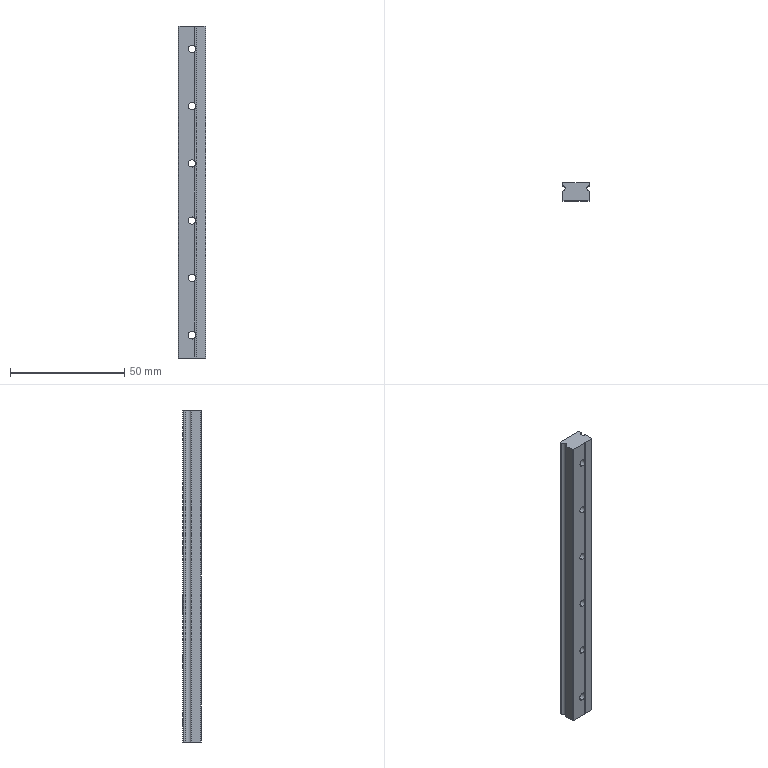Part | STEP file | MGN12C (slide rail) | 1 solid | 47 faces | box 12 x 8 x 145 mm | volume 12355 mm3 | cylinder 28 | plane 19 | commonest cylinder face diameters 6 x12 3.2 x10 2.5 x3 3.5 x2 0.6 x1